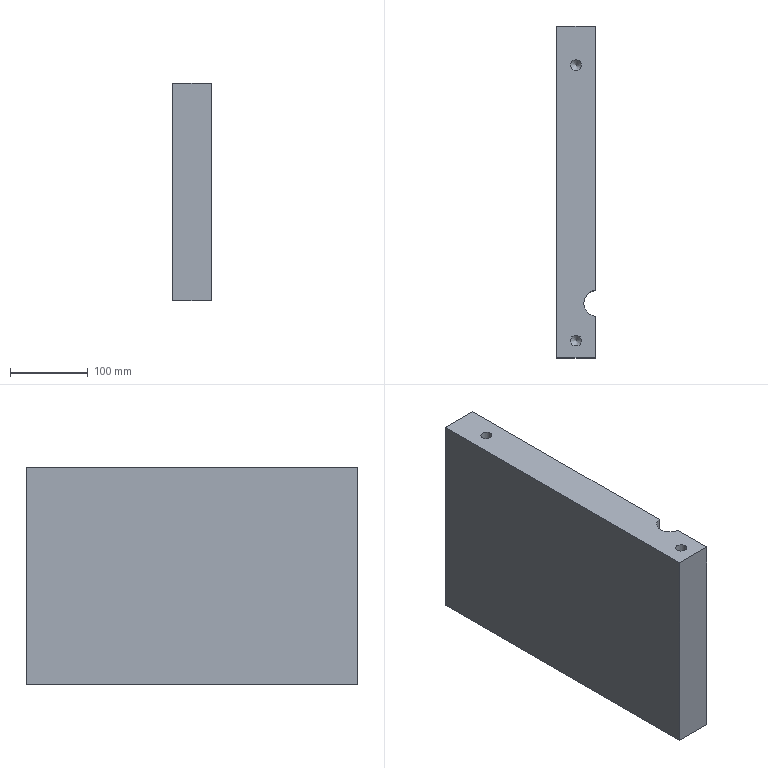Part | NX | features 29 2 | 1 solid | 16 faces | box 50 x 427.5 x 280.5 mm | volume 5862836 mm3 | plane 7 | cylinder 5 | cone 4 | commonest cylinder face diameters 14.1 x4 34 x1
STEP:
#1=CARTESIAN_POINT('',(857.05,622.,-493.5));
#2=VERTEX_POINT('',#1);
#3=CARTESIAN_POINT('',(850.,622.,-493.5));
#4=DIRECTION('',(0.,0.,1.));
#5=DIRECTION('',(1.,0.,0.));
#6=AXIS2_PLACEMENT_3D('',#3,#4,#5);
#7=CIRCLE('',#6,7.05);
#8=EDGE_CURVE('',#2,#2,#7,.T.);
#9=ORIENTED_EDGE('',*,*,#8,.T.);
#10=EDGE_LOOP('',(#9));
#11=FACE_BOUND('',#10,.T.);
#12=CARTESIAN_POINT('',(875.,331.882,-493.5));
#13=VERTEX_POINT('',#12);
#14=CARTESIAN_POINT('',(875.,672.5,-493.5));
#15=VERTEX_POINT('',#14);
#16=CARTESIAN_POINT('',(875.,193.,-493.5));
#17=DIRECTION('',(0.,1.,0.));
#18=VECTOR('',#17,1000.);
#19=LINE('',#16,#18);
#20=EDGE_CURVE('',#13,#15,#19,.T.);
#21=ORIENTED_EDGE('',*,*,#20,.F.);
#22=CARTESIAN_POINT('',(875.,298.118,-493.5));
#23=VERTEX_POINT('',#22);
#24=CARTESIAN_POINT('',(877.,315.,-493.5));
#25=DIRECTION('',(0.,0.,-1.));
#26=DIRECTION('',(-1.,0.,0.));
#27=AXIS2_PLACEMENT_3D('',#24,#25,#26);
#28=CIRCLE('',#27,17.);
#29=EDGE_CURVE('',#23,#13,#28,.T.);
#30=ORIENTED_EDGE('',*,*,#29,.F.);
#31=CARTESIAN_POINT('',(875.,245.,-493.5));
#32=VERTEX_POINT('',#31);
#33=CARTESIAN_POINT('',(875.,193.,-493.5));
#34=DIRECTION('',(0.,1.,0.));
#35=VECTOR('',#34,1000.);
#36=LINE('',#33,#35);
#37=EDGE_CURVE('',#32,#23,#36,.T.);
#38=ORIENTED_EDGE('',*,*,#37,.F.);
#39=CARTESIAN_POINT('',(825.,245.,-493.5));
#40=VERTEX_POINT('',#39);
#41=CARTESIAN_POINT('',(1625.,245.,-493.5));
#42=DIRECTION('',(-1.,0.,0.));
#43=VECTOR('',#42,1000.);
#44=LINE('',#41,#43);
#45=EDGE_CURVE('',#32,#40,#44,.T.);
#46=ORIENTED_EDGE('',*,*,#45,.T.);
#47=CARTESIAN_POINT('',(825.,672.5,-493.5));
#48=VERTEX_POINT('',#47);
#49=CARTESIAN_POINT('',(825.,193.,-493.5));
#50=DIRECTION('',(0.,-1.,0.));
#51=VECTOR('',#50,1000.);
#52=LINE('',#49,#51);
#53=EDGE_CURVE('',#48,#40,#52,.T.);
#54=ORIENTED_EDGE('',*,*,#53,.F.);
#55=CARTESIAN_POINT('',(1625.,672.5,-493.5));
#56=DIRECTION('',(1.,0.,0.));
#57=VECTOR('',#56,1000.);
#58=LINE('',#55,#57);
#59=EDGE_CURVE('',#48,#15,#58,.T.);
#60=ORIENTED_EDGE('',*,*,#59,.T.);
#61=EDGE_LOOP('',(#21,#30,#38,#46,#54,#60));
#62=FACE_BOUND('',#61,.T.);
#63=CARTESIAN_POINT('',(857.05,267.,-493.5));
#64=VERTEX_POINT('',#63);
#65=CARTESIAN_POINT('',(850.,267.,-493.5));
#66=DIRECTION('',(0.,0.,1.));
#67=DIRECTION('',(1.,0.,0.));
#68=AXIS2_PLACEMENT_3D('',#65,#66,#67);
#69=CIRCLE('',#68,7.05);
#70=EDGE_CURVE('',#64,#64,#69,.T.);
#71=ORIENTED_EDGE('',*,*,#70,.T.);
#72=EDGE_LOOP('',(#71));
#73=FACE_BOUND('',#72,.T.);
#74=CARTESIAN_POINT('',(1625.,0.,-493.5));
#75=DIRECTION('',(0.,0.,-1.));
#76=DIRECTION('',(1.,0.,0.));
#77=AXIS2_PLACEMENT_3D('',#74,#75,#76);
#78=PLANE('',#77);
#79=ADVANCED_FACE('',(#11,#62,#73),#78,.T.);
#80=CARTESIAN_POINT('',(857.05,622.,-213.));
#81=VERTEX_POINT('',#80);
#82=CARTESIAN_POINT('',(850.,622.,-213.));
#83=DIRECTION('',(0.,0.,-1.));
#84=DIRECTION('',(1.,0.,0.));
#85=AXIS2_PLACEMENT_3D('',#82,#83,#84);
#86=CIRCLE('',#85,7.05);
#87=EDGE_CURVE('',#81,#81,#86,.T.);
#88=ORIENTED_EDGE('',*,*,#87,.T.);
#89=EDGE_LOOP('',(#88));
#90=FACE_BOUND('',#89,.T.);
#91=CARTESIAN_POINT('',(875.,672.5,-213.));
#92=VERTEX_POINT('',#91);
#93=CARTESIAN_POINT('',(825.,672.5,-213.));
#94=VERTEX_POINT('',#93);
#95=CARTESIAN_POINT('',(1625.,672.5,-213.));
#96=DIRECTION('',(-1.,0.,0.));
#97=VECTOR('',#96,1000.);
#98=LINE('',#95,#97);
#99=EDGE_CURVE('',#92,#94,#98,.T.);
#100=ORIENTED_EDGE('',*,*,#99,.T.);
#101=CARTESIAN_POINT('',(825.,245.,-213.));
#102=VERTEX_POINT('',#101);
#103=CARTESIAN_POINT('',(825.,193.,-213.));
#104=DIRECTION('',(0.,1.,0.));
#105=VECTOR('',#104,1000.);
#106=LINE('',#103,#105);
#107=EDGE_CURVE('',#102,#94,#106,.T.);
#108=ORIENTED_EDGE('',*,*,#107,.F.);
#109=CARTESIAN_POINT('',(875.,245.,-213.));
#110=VERTEX_POINT('',#109);
#111=CARTESIAN_POINT('',(1625.,245.,-213.));
#112=DIRECTION('',(1.,0.,0.));
#113=VECTOR('',#112,1000.);
#114=LINE('',#111,#113);
#115=EDGE_CURVE('',#102,#110,#114,.T.);
#116=ORIENTED_EDGE('',*,*,#115,.T.);
#117=CARTESIAN_POINT('',(875.,298.118,-213.));
#118=VERTEX_POINT('',#117);
#119=CARTESIAN_POINT('',(875.,193.,-213.));
#120=DIRECTION('',(0.,-1.,0.));
#121=VECTOR('',#120,1000.);
#122=LINE('',#119,#121);
#123=EDGE_CURVE('',#118,#110,#122,.T.);
#124=ORIENTED_EDGE('',*,*,#123,.F.);
#125=CARTESIAN_POINT('',(875.,331.882,-213.));
#126=VERTEX_POINT('',#125);
#127=CARTESIAN_POINT('',(877.,315.,-213.));
#128=DIRECTION('',(0.,0.,1.));
#129=DIRECTION('',(1.,0.,0.));
#130=AXIS2_PLACEMENT_3D('',#127,#128,#129);
#131=CIRCLE('',#130,17.);
#132=EDGE_CURVE('',#126,#118,#131,.T.);
#133=ORIENTED_EDGE('',*,*,#132,.F.);
#134=CARTESIAN_POINT('',(875.,193.,-213.));
#135=DIRECTION('',(0.,-1.,0.));
#136=VECTOR('',#135,1000.);
#137=LINE('',#134,#136);
#138=EDGE_CURVE('',#92,#126,#137,.T.);
#139=ORIENTED_EDGE('',*,*,#138,.F.);
#140=EDGE_LOOP('',(#100,#108,#116,#124,#133,#139));
#141=FACE_BOUND('',#140,.T.);
#142=CARTESIAN_POINT('',(857.05,267.,-213.));
#143=VERTEX_POINT('',#142);
#144=CARTESIAN_POINT('',(850.,267.,-213.));
#145=DIRECTION('',(0.,0.,-1.));
#146=DIRECTION('',(1.,0.,0.));
#147=AXIS2_PLACEMENT_3D('',#144,#145,#146);
#148=CIRCLE('',#147,7.05);
#149=EDGE_CURVE('',#143,#143,#148,.T.);
#150=ORIENTED_EDGE('',*,*,#149,.T.);
#151=EDGE_LOOP('',(#150));
#152=FACE_BOUND('',#151,.T.);
#153=CARTESIAN_POINT('',(1625.,0.,-213.));
#154=DIRECTION('',(0.,0.,1.));
#155=DIRECTION('',(-1.,0.,0.));
#156=AXIS2_PLACEMENT_3D('',#153,#154,#155);
#157=PLANE('',#156);
#158=ADVANCED_FACE('',(#90,#141,#152),#157,.T.);
#159=ORIENTED_EDGE('',*,*,#138,.T.);
#160=CARTESIAN_POINT('',(875.,331.882,-774.));
#161=DIRECTION('',(0.,0.,-1.));
#162=VECTOR('',#161,1000.);
#163=LINE('',#160,#162);
#164=EDGE_CURVE('',#126,#13,#163,.T.);
#165=ORIENTED_EDGE('',*,*,#164,.T.);
#166=ORIENTED_EDGE('',*,*,#20,.T.);
#167=CARTESIAN_POINT('',(875.,672.5,-205.5));
#168=DIRECTION('',(0.,0.,1.));
#169=VECTOR('',#168,1000.);
#170=LINE('',#167,#169);
#171=EDGE_CURVE('',#15,#92,#170,.T.);
#172=ORIENTED_EDGE('',*,*,#171,.T.);
#173=EDGE_LOOP('',(#159,#165,#166,#172));
#174=FACE_BOUND('',#173,.T.);
#175=CARTESIAN_POINT('',(875.,193.,-205.5));
#176=DIRECTION('',(1.,0.,0.));
#177=DIRECTION('',(0.,0.,-1.));
#178=AXIS2_PLACEMENT_3D('',#175,#176,#177);
#179=PLANE('',#178);
#180=ADVANCED_FACE('',(#174),#179,.T.);
#181=ORIENTED_EDGE('',*,*,#37,.T.);
#182=CARTESIAN_POINT('',(875.,298.118,-493.5));
#183=DIRECTION('',(0.,0.,1.));
#184=VECTOR('',#183,1000.);
#185=LINE('',#182,#184);
#186=EDGE_CURVE('',#23,#118,#185,.T.);
#187=ORIENTED_EDGE('',*,*,#186,.T.);
#188=ORIENTED_EDGE('',*,*,#123,.T.);
#189=CARTESIAN_POINT('',(875.,245.,-205.5));
#190=DIRECTION('',(0.,0.,-1.));
#191=VECTOR('',#190,1000.);
#192=LINE('',#189,#191);
#193=EDGE_CURVE('',#110,#32,#192,.T.);
#194=ORIENTED_EDGE('',*,*,#193,.T.);
#195=EDGE_LOOP('',(#181,#187,#188,#194));
#196=FACE_BOUND('',#195,.T.);
#197=CARTESIAN_POINT('',(875.,193.,-205.5));
#198=DIRECTION('',(1.,0.,0.));
#199=DIRECTION('',(0.,0.,-1.));
#200=AXIS2_PLACEMENT_3D('',#197,#198,#199);
#201=PLANE('',#200);
#202=ADVANCED_FACE('',(#196),#201,.T.);
#203=ORIENTED_EDGE('',*,*,#115,.F.);
#204=CARTESIAN_POINT('',(825.,245.,-205.5));
#205=DIRECTION('',(0.,0.,1.));
#206=VECTOR('',#205,1000.);
#207=LINE('',#204,#206);
#208=EDGE_CURVE('',#40,#102,#207,.T.);
#209=ORIENTED_EDGE('',*,*,#208,.F.);
#210=ORIENTED_EDGE('',*,*,#45,.F.);
#211=ORIENTED_EDGE('',*,*,#193,.F.);
#212=EDGE_LOOP('',(#203,#209,#210,#211));
#213=FACE_BOUND('',#212,.T.);
#214=CARTESIAN_POINT('',(765.,245.,-518.5));
#215=DIRECTION('',(0.,-1.,0.));
#216=DIRECTION('',(0.,0.,1.));
#217=AXIS2_PLACEMENT_3D('',#214,#215,#216);
#218=PLANE('',#217);
#219=ADVANCED_FACE('',(#213),#218,.T.);
#220=ORIENTED_EDGE('',*,*,#107,.T.);
#221=CARTESIAN_POINT('',(825.,672.5,-205.5));
#222=DIRECTION('',(0.,0.,-1.));
#223=VECTOR('',#222,1000.);
#224=LINE('',#221,#223);
#225=EDGE_CURVE('',#94,#48,#224,.T.);
#226=ORIENTED_EDGE('',*,*,#225,.T.);
#227=ORIENTED_EDGE('',*,*,#53,.T.);
#228=ORIENTED_EDGE('',*,*,#208,.T.);
#229=EDGE_LOOP('',(#220,#226,#227,#228));
#230=FACE_BOUND('',#229,.T.);
#231=CARTESIAN_POINT('',(825.,193.,-205.5));
#232=DIRECTION('',(-1.,0.,0.));
#233=DIRECTION('',(0.,0.,1.));
#234=AXIS2_PLACEMENT_3D('',#231,#232,#233);
#235=PLANE('',#234);
#236=ADVANCED_FACE('',(#230),#235,.T.);
#237=ORIENTED_EDGE('',*,*,#99,.F.);
#238=ORIENTED_EDGE('',*,*,#171,.F.);
#239=ORIENTED_EDGE('',*,*,#59,.F.);
#240=ORIENTED_EDGE('',*,*,#225,.F.);
#241=EDGE_LOOP('',(#237,#238,#239,#240));
#242=FACE_BOUND('',#241,.T.);
#243=CARTESIAN_POINT('',(302.5,672.5,91.));
#244=DIRECTION('',(0.,-1.,0.));
#245=DIRECTION('',(-1.,0.,0.));
#246=AXIS2_PLACEMENT_3D('',#243,#244,#245);
#247=PLANE('',#246);
#248=ADVANCED_FACE('',(#242),#247,.F.);
#249=ORIENTED_EDGE('',*,*,#132,.T.);
#250=ORIENTED_EDGE('',*,*,#186,.F.);
#251=ORIENTED_EDGE('',*,*,#29,.T.);
#252=ORIENTED_EDGE('',*,*,#164,.F.);
#253=EDGE_LOOP('',(#249,#250,#251,#252));
#254=FACE_BOUND('',#253,.T.);
#255=CARTESIAN_POINT('',(877.,315.,-774.));
#256=DIRECTION('',(0.,0.,1.));
#257=DIRECTION('',(-1.,0.,0.));
#258=AXIS2_PLACEMENT_3D('',#255,#256,#257);
#259=CYLINDRICAL_SURFACE('',#258,17.);
#260=ADVANCED_FACE('',(#254),#259,.F.);
#261=CARTESIAN_POINT('',(842.95,622.,-249.95));
#262=VERTEX_POINT('',#261);
#263=CARTESIAN_POINT('',(850.,622.,-249.95));
#264=DIRECTION('',(0.,0.,-1.));
#265=DIRECTION('',(-1.,0.,0.));
#266=AXIS2_PLACEMENT_3D('',#263,#264,#265);
#267=CIRCLE('',#266,7.05);
#268=EDGE_CURVE('',#262,#262,#267,.T.);
#269=ORIENTED_EDGE('',*,*,#268,.T.);
#270=EDGE_LOOP('',(#269));
#271=FACE_BOUND('',#270,.T.);
#272=ORIENTED_EDGE('',*,*,#87,.F.);
#273=EDGE_LOOP('',(#272));
#274=FACE_BOUND('',#273,.T.);
#275=CARTESIAN_POINT('',(850.,622.,-213.));
#276=DIRECTION('',(0.,0.,-1.));
#277=DIRECTION('',(-1.,0.,0.));
#278=AXIS2_PLACEMENT_3D('',#275,#276,#277);
#279=CYLINDRICAL_SURFACE('',#278,7.05);
#280=ADVANCED_FACE('',(#271,#274),#279,.F.);
#281=CARTESIAN_POINT('',(850.,622.,-257.));
#282=VERTEX_POINT('',#281);
#283=VERTEX_LOOP('',#282);
#284=FACE_BOUND('',#283,.T.);
#285=ORIENTED_EDGE('',*,*,#268,.F.);
#286=EDGE_LOOP('',(#285));
#287=FACE_BOUND('',#286,.T.);
#288=CARTESIAN_POINT('',(850.,622.,-249.95));
#289=DIRECTION('',(0.,0.,1.));
#290=DIRECTION('',(-1.,0.,0.));
#291=AXIS2_PLACEMENT_3D('',#288,#289,#290);
#292=CONICAL_SURFACE('',#291,7.05,0.7854);
#293=ADVANCED_FACE('',(#284,#287),#292,.F.);
#294=CARTESIAN_POINT('',(842.95,267.,-249.95));
#295=VERTEX_POINT('',#294);
#296=CARTESIAN_POINT('',(850.,267.,-249.95));
#297=DIRECTION('',(0.,0.,-1.));
#298=DIRECTION('',(-1.,0.,0.));
#299=AXIS2_PLACEMENT_3D('',#296,#297,#298);
#300=CIRCLE('',#299,7.05);
#301=EDGE_CURVE('',#295,#295,#300,.T.);
#302=ORIENTED_EDGE('',*,*,#301,.T.);
#303=EDGE_LOOP('',(#302));
#304=FACE_BOUND('',#303,.T.);
#305=ORIENTED_EDGE('',*,*,#149,.F.);
#306=EDGE_LOOP('',(#305));
#307=FACE_BOUND('',#306,.T.);
#308=CARTESIAN_POINT('',(850.,267.,-213.));
#309=DIRECTION('',(0.,0.,-1.));
#310=DIRECTION('',(-1.,0.,0.));
#311=AXIS2_PLACEMENT_3D('',#308,#309,#310);
#312=CYLINDRICAL_SURFACE('',#311,7.05);
#313=ADVANCED_FACE('',(#304,#307),#312,.F.);
#314=CARTESIAN_POINT('',(850.,267.,-257.));
#315=VERTEX_POINT('',#314);
#316=VERTEX_LOOP('',#315);
#317=FACE_BOUND('',#316,.T.);
#318=ORIENTED_EDGE('',*,*,#301,.F.);
#319=EDGE_LOOP('',(#318));
#320=FACE_BOUND('',#319,.T.);
#321=CARTESIAN_POINT('',(850.,267.,-249.95));
#322=DIRECTION('',(0.,0.,1.));
#323=DIRECTION('',(-1.,0.,0.));
#324=AXIS2_PLACEMENT_3D('',#321,#322,#323);
#325=CONICAL_SURFACE('',#324,7.05,0.7854);
#326=ADVANCED_FACE('',(#317,#320),#325,.F.);
#327=CARTESIAN_POINT('',(857.05,622.,-456.55));
#328=VERTEX_POINT('',#327);
#329=CARTESIAN_POINT('',(850.,622.,-456.55));
#330=DIRECTION('',(0.,0.,1.));
#331=DIRECTION('',(1.,0.,0.));
#332=AXIS2_PLACEMENT_3D('',#329,#330,#331);
#333=CIRCLE('',#332,7.05);
#334=EDGE_CURVE('',#328,#328,#333,.T.);
#335=ORIENTED_EDGE('',*,*,#334,.T.);
#336=EDGE_LOOP('',(#335));
#337=FACE_BOUND('',#336,.T.);
#338=ORIENTED_EDGE('',*,*,#8,.F.);
#339=EDGE_LOOP('',(#338));
#340=FACE_BOUND('',#339,.T.);
#341=CARTESIAN_POINT('',(850.,622.,-493.5));
#342=DIRECTION('',(0.,0.,1.));
#343=DIRECTION('',(-1.,0.,0.));
#344=AXIS2_PLACEMENT_3D('',#341,#342,#343);
#345=CYLINDRICAL_SURFACE('',#344,7.05);
#346=ADVANCED_FACE('',(#337,#340),#345,.F.);
#347=CARTESIAN_POINT('',(850.,622.,-449.5));
#348=VERTEX_POINT('',#347);
#349=VERTEX_LOOP('',#348);
#350=FACE_BOUND('',#349,.T.);
#351=ORIENTED_EDGE('',*,*,#334,.F.);
#352=EDGE_LOOP('',(#351));
#353=FACE_BOUND('',#352,.T.);
#354=CARTESIAN_POINT('',(850.,622.,-456.55));
#355=DIRECTION('',(0.,0.,-1.));
#356=DIRECTION('',(1.,0.,0.));
#357=AXIS2_PLACEMENT_3D('',#354,#355,#356);
#358=CONICAL_SURFACE('',#357,7.05,0.7854);
#359=ADVANCED_FACE('',(#350,#353),#358,.F.);
#360=CARTESIAN_POINT('',(857.05,267.,-456.55));
#361=VERTEX_POINT('',#360);
#362=CARTESIAN_POINT('',(850.,267.,-456.55));
#363=DIRECTION('',(0.,0.,1.));
#364=DIRECTION('',(1.,0.,0.));
#365=AXIS2_PLACEMENT_3D('',#362,#363,#364);
#366=CIRCLE('',#365,7.05);
#367=EDGE_CURVE('',#361,#361,#366,.T.);
#368=ORIENTED_EDGE('',*,*,#367,.T.);
#369=EDGE_LOOP('',(#368));
#370=FACE_BOUND('',#369,.T.);
#371=ORIENTED_EDGE('',*,*,#70,.F.);
#372=EDGE_LOOP('',(#371));
#373=FACE_BOUND('',#372,.T.);
#374=CARTESIAN_POINT('',(850.,267.,-493.5));
#375=DIRECTION('',(0.,0.,1.));
#376=DIRECTION('',(-1.,0.,0.));
#377=AXIS2_PLACEMENT_3D('',#374,#375,#376);
#378=CYLINDRICAL_SURFACE('',#377,7.05);
#379=ADVANCED_FACE('',(#370,#373),#378,.F.);
#380=CARTESIAN_POINT('',(850.,267.,-449.5));
#381=VERTEX_POINT('',#380);
#382=VERTEX_LOOP('',#381);
#383=FACE_BOUND('',#382,.T.);
#384=ORIENTED_EDGE('',*,*,#367,.F.);
#385=EDGE_LOOP('',(#384));
#386=FACE_BOUND('',#385,.T.);
#387=CARTESIAN_POINT('',(850.,267.,-456.55));
#388=DIRECTION('',(0.,0.,-1.));
#389=DIRECTION('',(1.,0.,0.));
#390=AXIS2_PLACEMENT_3D('',#387,#388,#389);
#391=CONICAL_SURFACE('',#390,7.05,0.7854);
#392=ADVANCED_FACE('',(#383,#386),#391,.F.);
#393=CLOSED_SHELL('',(#79,#158,#180,#202,#219,#236,#248,#260,#280,#293,#313,#326,#346,#359,#379,#392));
#394=MANIFOLD_SOLID_BREP('',#393);
#395=(LENGTH_UNIT()NAMED_UNIT(*)SI_UNIT(.MILLI.,.METRE.));
#396=UNCERTAINTY_MEASURE_WITH_UNIT(LENGTH_MEASURE(0.00001),#395,'','');
#397=(NAMED_UNIT(*)PLANE_ANGLE_UNIT()SI_UNIT($,.RADIAN.));
#398=(NAMED_UNIT(*)SI_UNIT($,.STERADIAN.)SOLID_ANGLE_UNIT());
#399=(GEOMETRIC_REPRESENTATION_CONTEXT(3)GLOBAL_UNCERTAINTY_ASSIGNED_CONTEXT((#396))GLOBAL_UNIT_ASSIGNED_CONTEXT((#395,#397,#398))REPRESENTATION_CONTEXT('',''));
#400=ADVANCED_BREP_SHAPE_REPRESENTATION('',(#394),#399);